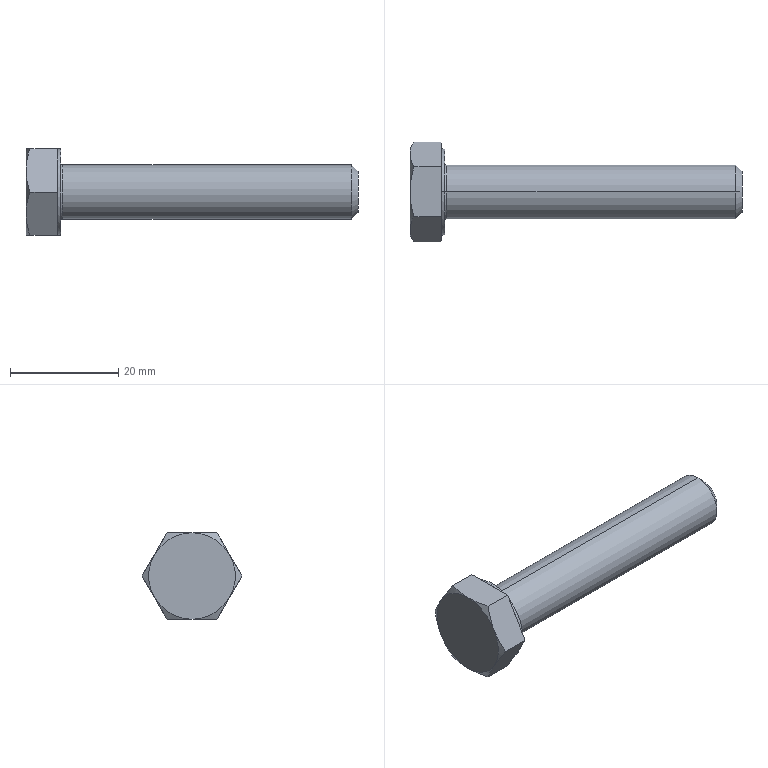Part | SolidWorks | features RevCut 4, Chamfer 1, Extrusion 1, Fillet 1, LPattern 1, Revolution 1 | 1 solid | 35 faces | box 61.4 x 18.475 x 16 mm | volume 5702 mm3 | plane 15 | cone 14 | cylinder 4 | torus 2 | commonest cylinder face diameters 10 x2 16 x2
STEP:
#1=CARTESIAN_POINT('',(6.8,0.,5.));
#2=VERTEX_POINT('',#1);
#3=CARTESIAN_POINT('',(6.8,0.,-5.));
#4=VERTEX_POINT('',#3);
#5=CARTESIAN_POINT('',(6.8,0.,0.));
#6=DIRECTION('',(1.,0.,0.));
#7=DIRECTION('',(0.,0.,-1.));
#8=AXIS2_PLACEMENT_3D('',#5,#6,#7);
#9=CIRCLE('',#8,5.);
#10=EDGE_CURVE('',#2,#4,#9,.T.);
#11=ORIENTED_EDGE('',*,*,#10,.F.);
#12=CARTESIAN_POINT('',(6.4,0.,5.4));
#13=VERTEX_POINT('',#12);
#14=CARTESIAN_POINT('',(6.8,0.,5.4));
#15=DIRECTION('',(0.,1.,0.));
#16=DIRECTION('',(0.,0.,1.));
#17=AXIS2_PLACEMENT_3D('',#14,#15,#16);
#18=CIRCLE('',#17,0.4);
#19=EDGE_CURVE('',#2,#13,#18,.T.);
#20=ORIENTED_EDGE('',*,*,#19,.T.);
#21=CARTESIAN_POINT('',(6.4,0.,-5.4));
#22=VERTEX_POINT('',#21);
#23=CARTESIAN_POINT('',(6.4,0.,0.));
#24=DIRECTION('',(-1.,0.,0.));
#25=DIRECTION('',(0.,0.,-1.));
#26=AXIS2_PLACEMENT_3D('',#23,#24,#25);
#27=CIRCLE('',#26,5.4);
#28=EDGE_CURVE('',#22,#13,#27,.T.);
#29=ORIENTED_EDGE('',*,*,#28,.F.);
#30=CARTESIAN_POINT('',(6.8,0.,-5.4));
#31=DIRECTION('',(0.,-1.,0.));
#32=DIRECTION('',(0.,0.,-1.));
#33=AXIS2_PLACEMENT_3D('',#30,#31,#32);
#34=CIRCLE('',#33,0.4);
#35=EDGE_CURVE('',#4,#22,#34,.T.);
#36=ORIENTED_EDGE('',*,*,#35,.F.);
#37=EDGE_LOOP('',(#11,#20,#29,#36));
#38=FACE_OUTER_BOUND('',#37,.T.);
#39=CARTESIAN_POINT('',(6.8,0.,0.));
#40=DIRECTION('',(1.,0.,0.));
#41=DIRECTION('',(0.,0.,-1.));
#42=AXIS2_PLACEMENT_3D('',#39,#40,#41);
#43=TOROIDAL_SURFACE('',#42,5.4,0.4);
#44=ADVANCED_FACE('',(#38),#43,.F.);
#45=CARTESIAN_POINT('',(61.4,0.,-3.8));
#46=VERTEX_POINT('',#45);
#47=CARTESIAN_POINT('',(61.4,0.,3.8));
#48=VERTEX_POINT('',#47);
#49=CARTESIAN_POINT('',(61.4,0.,0.));
#50=DIRECTION('',(1.,0.,0.));
#51=DIRECTION('',(0.,0.,1.));
#52=AXIS2_PLACEMENT_3D('',#49,#50,#51);
#53=CIRCLE('',#52,3.8);
#54=EDGE_CURVE('',#46,#48,#53,.T.);
#55=ORIENTED_EDGE('',*,*,#54,.F.);
#56=CARTESIAN_POINT('',(60.2,0.,-5.));
#57=VERTEX_POINT('',#56);
#58=CARTESIAN_POINT('',(60.2,0.,-5.));
#59=DIRECTION('',(-0.7071,0.,-0.7071));
#60=VECTOR('',#59,1000.);
#61=LINE('',#58,#60);
#62=EDGE_CURVE('',#46,#57,#61,.T.);
#63=ORIENTED_EDGE('',*,*,#62,.T.);
#64=CARTESIAN_POINT('',(60.2,0.,5.));
#65=VERTEX_POINT('',#64);
#66=CARTESIAN_POINT('',(60.2,0.,0.));
#67=DIRECTION('',(-1.,0.,0.));
#68=DIRECTION('',(0.,0.,1.));
#69=AXIS2_PLACEMENT_3D('',#66,#67,#68);
#70=CIRCLE('',#69,5.);
#71=EDGE_CURVE('',#65,#57,#70,.T.);
#72=ORIENTED_EDGE('',*,*,#71,.F.);
#73=CARTESIAN_POINT('',(60.2,0.,5.));
#74=DIRECTION('',(-0.7071,0.,0.7071));
#75=VECTOR('',#74,1000.);
#76=LINE('',#73,#75);
#77=EDGE_CURVE('',#48,#65,#76,.T.);
#78=ORIENTED_EDGE('',*,*,#77,.F.);
#79=EDGE_LOOP('',(#55,#63,#72,#78));
#80=FACE_OUTER_BOUND('',#79,.T.);
#81=CARTESIAN_POINT('',(60.2,0.,0.));
#82=DIRECTION('',(-1.,0.,0.));
#83=DIRECTION('',(0.,0.,1.));
#84=AXIS2_PLACEMENT_3D('',#81,#82,#83);
#85=CONICAL_SURFACE('',#84,5.,0.7854);
#86=ADVANCED_FACE('',(#80),#85,.T.);
#87=ORIENTED_EDGE('',*,*,#71,.T.);
#88=CARTESIAN_POINT('',(0.,0.,-5.));
#89=DIRECTION('',(-1.,0.,0.));
#90=VECTOR('',#89,1000.);
#91=LINE('',#88,#90);
#92=EDGE_CURVE('',#57,#4,#91,.T.);
#93=ORIENTED_EDGE('',*,*,#92,.T.);
#94=CARTESIAN_POINT('',(6.8,0.,0.));
#95=DIRECTION('',(1.,0.,0.));
#96=DIRECTION('',(0.,0.,-1.));
#97=AXIS2_PLACEMENT_3D('',#94,#95,#96);
#98=CIRCLE('',#97,5.);
#99=EDGE_CURVE('',#4,#2,#98,.T.);
#100=ORIENTED_EDGE('',*,*,#99,.T.);
#101=CARTESIAN_POINT('',(0.,0.,5.));
#102=DIRECTION('',(-1.,0.,0.));
#103=VECTOR('',#102,1000.);
#104=LINE('',#101,#103);
#105=EDGE_CURVE('',#65,#2,#104,.T.);
#106=ORIENTED_EDGE('',*,*,#105,.F.);
#107=EDGE_LOOP('',(#87,#93,#100,#106));
#108=FACE_OUTER_BOUND('',#107,.T.);
#109=CARTESIAN_POINT('',(0.,0.,0.));
#110=DIRECTION('',(-1.,0.,0.));
#111=DIRECTION('',(0.,0.,1.));
#112=AXIS2_PLACEMENT_3D('',#109,#110,#111);
#113=CYLINDRICAL_SURFACE('',#112,5.);
#114=ADVANCED_FACE('',(#108),#113,.T.);
#115=CARTESIAN_POINT('',(6.4,0.,-8.));
#116=VERTEX_POINT('',#115);
#117=CARTESIAN_POINT('',(6.4,0.,8.));
#118=VERTEX_POINT('',#117);
#119=CARTESIAN_POINT('',(6.4,0.,0.));
#120=DIRECTION('',(1.,0.,0.));
#121=DIRECTION('',(0.,0.,-1.));
#122=AXIS2_PLACEMENT_3D('',#119,#120,#121);
#123=CIRCLE('',#122,8.);
#124=EDGE_CURVE('',#116,#118,#123,.T.);
#125=ORIENTED_EDGE('',*,*,#124,.F.);
#126=CARTESIAN_POINT('',(5.8,0.,-8.));
#127=VERTEX_POINT('',#126);
#128=CARTESIAN_POINT('',(0.,0.,-8.));
#129=DIRECTION('',(-1.,0.,0.));
#130=VECTOR('',#129,1000.);
#131=LINE('',#128,#130);
#132=EDGE_CURVE('',#116,#127,#131,.T.);
#133=ORIENTED_EDGE('',*,*,#132,.T.);
#134=CARTESIAN_POINT('',(5.8,6.928,-4.));
#135=VERTEX_POINT('',#134);
#136=CARTESIAN_POINT('',(5.8,0.,0.));
#137=DIRECTION('',(-1.,0.,0.));
#138=DIRECTION('',(0.,0.,1.));
#139=AXIS2_PLACEMENT_3D('',#136,#137,#138);
#140=CIRCLE('',#139,8.);
#141=EDGE_CURVE('',#135,#127,#140,.T.);
#142=ORIENTED_EDGE('',*,*,#141,.F.);
#143=CARTESIAN_POINT('',(5.8,6.928,4.));
#144=VERTEX_POINT('',#143);
#145=CARTESIAN_POINT('',(5.8,0.,0.));
#146=DIRECTION('',(-1.,0.,0.));
#147=DIRECTION('',(0.,0.,1.));
#148=AXIS2_PLACEMENT_3D('',#145,#146,#147);
#149=CIRCLE('',#148,8.);
#150=EDGE_CURVE('',#144,#135,#149,.T.);
#151=ORIENTED_EDGE('',*,*,#150,.F.);
#152=CARTESIAN_POINT('',(5.8,0.,8.));
#153=VERTEX_POINT('',#152);
#154=CARTESIAN_POINT('',(5.8,0.,0.));
#155=DIRECTION('',(-1.,0.,0.));
#156=DIRECTION('',(0.,0.,1.));
#157=AXIS2_PLACEMENT_3D('',#154,#155,#156);
#158=CIRCLE('',#157,8.);
#159=EDGE_CURVE('',#153,#144,#158,.T.);
#160=ORIENTED_EDGE('',*,*,#159,.F.);
#161=CARTESIAN_POINT('',(0.,0.,8.));
#162=DIRECTION('',(-1.,0.,0.));
#163=VECTOR('',#162,1000.);
#164=LINE('',#161,#163);
#165=EDGE_CURVE('',#118,#153,#164,.T.);
#166=ORIENTED_EDGE('',*,*,#165,.F.);
#167=EDGE_LOOP('',(#125,#133,#142,#151,#160,#166));
#168=FACE_OUTER_BOUND('',#167,.T.);
#169=CARTESIAN_POINT('',(0.,0.,0.));
#170=DIRECTION('',(-1.,0.,0.));
#171=DIRECTION('',(0.,0.,1.));
#172=AXIS2_PLACEMENT_3D('',#169,#170,#171);
#173=CYLINDRICAL_SURFACE('',#172,8.);
#174=ADVANCED_FACE('',(#168),#173,.T.);
#175=CARTESIAN_POINT('',(5.8,4.824,-7.644));
#176=VERTEX_POINT('',#175);
#177=CARTESIAN_POINT('',(5.8,4.619,-8.));
#178=DIRECTION('',(0.,0.5,0.866));
#179=VECTOR('',#178,1000.);
#180=LINE('',#177,#179);
#181=EDGE_CURVE('',#176,#135,#180,.T.);
#182=ORIENTED_EDGE('',*,*,#181,.F.);
#183=CARTESIAN_POINT('',(5.685,4.619,-8.));
#184=VERTEX_POINT('',#183);
#185=CARTESIAN_POINT('',(5.685,4.619,-8.));
#186=CARTESIAN_POINT('',(5.725,4.687,-7.882));
#187=CARTESIAN_POINT('',(5.763,4.756,-7.763));
#188=CARTESIAN_POINT('',(5.8,4.824,-7.644));
#189=B_SPLINE_CURVE_WITH_KNOTS('',3,(#185,#186,#187,#188),.UNSPECIFIED.,.F.,.F.,(4,4),(0.000000238,0.0004231),.UNSPECIFIED.);
#190=EDGE_CURVE('',#184,#176,#189,.T.);
#191=ORIENTED_EDGE('',*,*,#190,.F.);
#192=CARTESIAN_POINT('',(0.7145,4.619,-8.));
#193=VERTEX_POINT('',#192);
#194=CARTESIAN_POINT('',(6.4,4.619,-8.));
#195=DIRECTION('',(-1.,0.,0.));
#196=VECTOR('',#195,1000.);
#197=LINE('',#194,#196);
#198=EDGE_CURVE('',#184,#193,#197,.T.);
#199=ORIENTED_EDGE('',*,*,#198,.T.);
#200=CARTESIAN_POINT('',(0.,6.928,-4.));
#201=VERTEX_POINT('',#200);
#202=CARTESIAN_POINT('',(0.,6.928,-4.));
#203=CARTESIAN_POINT('',(0.,6.732,-4.339));
#204=CARTESIAN_POINT('',(0.01689,6.535,-4.68));
#205=CARTESIAN_POINT('',(0.08225,6.146,-5.355));
#206=CARTESIAN_POINT('',(0.1307,5.952,-5.69));
#207=CARTESIAN_POINT('',(0.3174,5.376,-6.689));
#208=CARTESIAN_POINT('',(0.497,4.996,-7.347));
#209=CARTESIAN_POINT('',(0.7145,4.619,-8.));
#210=B_SPLINE_CURVE_WITH_KNOTS('',3,(#202,#203,#204,#205,#206,#207,#208,#209),.UNSPECIFIED.,.F.,.F.,(4,2,2,4),(0.004674,0.005838,0.007002,0.00933),.UNSPECIFIED.);
#211=EDGE_CURVE('',#201,#193,#210,.T.);
#212=ORIENTED_EDGE('',*,*,#211,.F.);
#213=CARTESIAN_POINT('',(0.7145,9.238,0.));
#214=VERTEX_POINT('',#213);
#215=CARTESIAN_POINT('',(0.7145,9.238,0.));
#216=CARTESIAN_POINT('',(0.4964,8.86,-0.6543));
#217=CARTESIAN_POINT('',(0.3167,8.479,-1.313));
#218=CARTESIAN_POINT('',(0.0681,7.71,-2.646));
#219=CARTESIAN_POINT('',(0.,7.322,-3.319));
#220=CARTESIAN_POINT('',(0.,6.928,-4.));
#221=B_SPLINE_CURVE_WITH_KNOTS('',3,(#215,#216,#217,#218,#219,#220),.UNSPECIFIED.,.F.,.F.,(4,2,4),(0.000000238,0.002337,0.004674),.UNSPECIFIED.);
#222=EDGE_CURVE('',#214,#201,#221,.T.);
#223=ORIENTED_EDGE('',*,*,#222,.F.);
#224=CARTESIAN_POINT('',(5.685,9.238,0.));
#225=VERTEX_POINT('',#224);
#226=CARTESIAN_POINT('',(6.4,9.238,0.));
#227=DIRECTION('',(-1.,0.,0.));
#228=VECTOR('',#227,1000.);
#229=LINE('',#226,#228);
#230=EDGE_CURVE('',#225,#214,#229,.T.);
#231=ORIENTED_EDGE('',*,*,#230,.F.);
#232=CARTESIAN_POINT('',(5.8,9.032,-0.3557));
#233=VERTEX_POINT('',#232);
#234=CARTESIAN_POINT('',(5.8,9.032,-0.3557));
#235=CARTESIAN_POINT('',(5.763,9.101,-0.237));
#236=CARTESIAN_POINT('',(5.725,9.169,-0.1184));
#237=CARTESIAN_POINT('',(5.685,9.238,0.));
#238=B_SPLINE_CURVE_WITH_KNOTS('',3,(#234,#235,#236,#237),.UNSPECIFIED.,.F.,.F.,(4,4),(0.008907,0.00933),.UNSPECIFIED.);
#239=EDGE_CURVE('',#233,#225,#238,.T.);
#240=ORIENTED_EDGE('',*,*,#239,.F.);
#241=CARTESIAN_POINT('',(5.8,4.619,-8.));
#242=DIRECTION('',(0.,0.5,0.866));
#243=VECTOR('',#242,1000.);
#244=LINE('',#241,#243);
#245=EDGE_CURVE('',#135,#233,#244,.T.);
#246=ORIENTED_EDGE('',*,*,#245,.F.);
#247=EDGE_LOOP('',(#182,#191,#199,#212,#223,#231,#240,#246));
#248=FACE_OUTER_BOUND('',#247,.T.);
#249=CARTESIAN_POINT('',(6.4,4.619,-8.));
#250=DIRECTION('',(0.,-0.866,0.5));
#251=DIRECTION('',(0.,-0.5,-0.866));
#252=AXIS2_PLACEMENT_3D('',#249,#250,#251);
#253=PLANE('',#252);
#254=ADVANCED_FACE('',(#248),#253,.F.);
#255=CARTESIAN_POINT('',(5.8,9.032,0.3557));
#256=VERTEX_POINT('',#255);
#257=CARTESIAN_POINT('',(5.8,9.238,0.));
#258=DIRECTION('',(0.,-0.5,0.866));
#259=VECTOR('',#258,1000.);
#260=LINE('',#257,#259);
#261=EDGE_CURVE('',#256,#144,#260,.T.);
#262=ORIENTED_EDGE('',*,*,#261,.F.);
#263=CARTESIAN_POINT('',(5.685,9.238,0.));
#264=CARTESIAN_POINT('',(5.725,9.169,0.1184));
#265=CARTESIAN_POINT('',(5.763,9.101,0.237));
#266=CARTESIAN_POINT('',(5.8,9.032,0.3557));
#267=B_SPLINE_CURVE_WITH_KNOTS('',3,(#263,#264,#265,#266),.UNSPECIFIED.,.F.,.F.,(4,4),(0.000000238,0.0004231),.UNSPECIFIED.);
#268=EDGE_CURVE('',#225,#256,#267,.T.);
#269=ORIENTED_EDGE('',*,*,#268,.F.);
#270=ORIENTED_EDGE('',*,*,#230,.T.);
#271=CARTESIAN_POINT('',(0.,6.928,4.));
#272=VERTEX_POINT('',#271);
#273=CARTESIAN_POINT('',(0.,6.928,4.));
#274=CARTESIAN_POINT('',(0.,7.124,3.661));
#275=CARTESIAN_POINT('',(0.01689,7.321,3.32));
#276=CARTESIAN_POINT('',(0.08225,7.711,2.645));
#277=CARTESIAN_POINT('',(0.1307,7.904,2.31));
#278=CARTESIAN_POINT('',(0.3174,8.481,1.311));
#279=CARTESIAN_POINT('',(0.497,8.861,0.6527));
#280=CARTESIAN_POINT('',(0.7145,9.238,0.));
#281=B_SPLINE_CURVE_WITH_KNOTS('',3,(#273,#274,#275,#276,#277,#278,#279,#280),.UNSPECIFIED.,.F.,.F.,(4,2,2,4),(0.004674,0.005838,0.007002,0.00933),.UNSPECIFIED.);
#282=EDGE_CURVE('',#272,#214,#281,.T.);
#283=ORIENTED_EDGE('',*,*,#282,.F.);
#284=CARTESIAN_POINT('',(0.7145,4.619,8.));
#285=VERTEX_POINT('',#284);
#286=CARTESIAN_POINT('',(0.7145,4.619,8.));
#287=CARTESIAN_POINT('',(0.4964,4.997,7.346));
#288=CARTESIAN_POINT('',(0.3167,5.377,6.687));
#289=CARTESIAN_POINT('',(0.0681,6.146,5.354));
#290=CARTESIAN_POINT('',(0.,6.535,4.681));
#291=CARTESIAN_POINT('',(0.,6.928,4.));
#292=B_SPLINE_CURVE_WITH_KNOTS('',3,(#286,#287,#288,#289,#290,#291),.UNSPECIFIED.,.F.,.F.,(4,2,4),(0.000000238,0.002337,0.004674),.UNSPECIFIED.);
#293=EDGE_CURVE('',#285,#272,#292,.T.);
#294=ORIENTED_EDGE('',*,*,#293,.F.);
#295=CARTESIAN_POINT('',(5.685,4.619,8.));
#296=VERTEX_POINT('',#295);
#297=CARTESIAN_POINT('',(6.4,4.619,8.));
#298=DIRECTION('',(-1.,0.,0.));
#299=VECTOR('',#298,1000.);
#300=LINE('',#297,#299);
#301=EDGE_CURVE('',#296,#285,#300,.T.);
#302=ORIENTED_EDGE('',*,*,#301,.F.);
#303=CARTESIAN_POINT('',(5.8,4.824,7.644));
#304=VERTEX_POINT('',#303);
#305=CARTESIAN_POINT('',(5.8,4.824,7.644));
#306=CARTESIAN_POINT('',(5.763,4.756,7.763));
#307=CARTESIAN_POINT('',(5.725,4.687,7.882));
#308=CARTESIAN_POINT('',(5.685,4.619,8.));
#309=B_SPLINE_CURVE_WITH_KNOTS('',3,(#305,#306,#307,#308),.UNSPECIFIED.,.F.,.F.,(4,4),(0.008907,0.00933),.UNSPECIFIED.);
#310=EDGE_CURVE('',#304,#296,#309,.T.);
#311=ORIENTED_EDGE('',*,*,#310,.F.);
#312=CARTESIAN_POINT('',(5.8,9.238,0.));
#313=DIRECTION('',(0.,-0.5,0.866));
#314=VECTOR('',#313,1000.);
#315=LINE('',#312,#314);
#316=EDGE_CURVE('',#144,#304,#315,.T.);
#317=ORIENTED_EDGE('',*,*,#316,.F.);
#318=EDGE_LOOP('',(#262,#269,#270,#283,#294,#302,#311,#317));
#319=FACE_OUTER_BOUND('',#318,.T.);
#320=CARTESIAN_POINT('',(6.4,9.238,0.));
#321=DIRECTION('',(0.,-0.866,-0.5));
#322=DIRECTION('',(0.,0.5,-0.866));
#323=AXIS2_PLACEMENT_3D('',#320,#321,#322);
#324=PLANE('',#323);
#325=ADVANCED_FACE('',(#319),#324,.F.);
#326=CARTESIAN_POINT('',(5.8,4.208,8.));
#327=VERTEX_POINT('',#326);
#328=CARTESIAN_POINT('',(5.8,4.619,8.));
#329=DIRECTION('',(0.,-1.,0.));
#330=VECTOR('',#329,1000.);
#331=LINE('',#328,#330);
#332=EDGE_CURVE('',#327,#153,#331,.T.);
#333=ORIENTED_EDGE('',*,*,#332,.F.);
#334=CARTESIAN_POINT('',(5.685,4.619,8.));
#335=CARTESIAN_POINT('',(5.725,4.482,8.));
#336=CARTESIAN_POINT('',(5.763,4.345,8.));
#337=CARTESIAN_POINT('',(5.8,4.208,8.));
#338=B_SPLINE_CURVE_WITH_KNOTS('',3,(#334,#335,#336,#337),.UNSPECIFIED.,.F.,.F.,(4,4),(0.02285,0.02328),.UNSPECIFIED.);
#339=EDGE_CURVE('',#296,#327,#338,.T.);
#340=ORIENTED_EDGE('',*,*,#339,.F.);
#341=ORIENTED_EDGE('',*,*,#301,.T.);
#342=CARTESIAN_POINT('',(0.,0.,8.));
#343=VERTEX_POINT('',#342);
#344=CARTESIAN_POINT('',(0.,0.,8.));
#345=CARTESIAN_POINT('',(0.,0.3913,8.));
#346=CARTESIAN_POINT('',(0.01678,0.7854,8.));
#347=CARTESIAN_POINT('',(0.08286,1.571,8.));
#348=CARTESIAN_POINT('',(0.1318,1.96,8.));
#349=CARTESIAN_POINT('',(0.3194,3.115,8.));
#350=CARTESIAN_POINT('',(0.4988,3.872,8.));
#351=CARTESIAN_POINT('',(0.7145,4.619,8.));
#352=B_SPLINE_CURVE_WITH_KNOTS('',3,(#344,#345,#346,#347,#348,#349,#350,#351),.UNSPECIFIED.,.F.,.F.,(4,2,2,4),(0.01337,0.01454,0.01571,0.01805),.UNSPECIFIED.);
#353=EDGE_CURVE('',#343,#285,#352,.T.);
#354=ORIENTED_EDGE('',*,*,#353,.F.);
#355=CARTESIAN_POINT('',(0.7145,-4.619,8.));
#356=VERTEX_POINT('',#355);
#357=CARTESIAN_POINT('',(0.7145,-4.619,8.));
#358=CARTESIAN_POINT('',(0.4973,-3.866,8.));
#359=CARTESIAN_POINT('',(0.3158,-3.098,8.));
#360=CARTESIAN_POINT('',(0.0673,-1.557,8.));
#361=CARTESIAN_POINT('',(0.,-0.7819,8.));
#362=CARTESIAN_POINT('',(0.,0.,8.));
#363=B_SPLINE_CURVE_WITH_KNOTS('',3,(#357,#358,#359,#360,#361,#362),.UNSPECIFIED.,.F.,.F.,(4,2,4),(0.00869,0.01103,0.01337),.UNSPECIFIED.);
#364=EDGE_CURVE('',#356,#343,#363,.T.);
#365=ORIENTED_EDGE('',*,*,#364,.F.);
#366=CARTESIAN_POINT('',(5.685,-4.619,8.));
#367=VERTEX_POINT('',#366);
#368=CARTESIAN_POINT('',(6.4,-4.619,8.));
#369=DIRECTION('',(-1.,0.,0.));
#370=VECTOR('',#369,1000.);
#371=LINE('',#368,#370);
#372=EDGE_CURVE('',#367,#356,#371,.T.);
#373=ORIENTED_EDGE('',*,*,#372,.F.);
#374=CARTESIAN_POINT('',(5.8,-4.208,8.));
#375=VERTEX_POINT('',#374);
#376=CARTESIAN_POINT('',(5.8,-4.208,8.));
#377=CARTESIAN_POINT('',(5.763,-4.345,8.));
#378=CARTESIAN_POINT('',(5.725,-4.482,8.));
#379=CARTESIAN_POINT('',(5.685,-4.619,8.));
#380=B_SPLINE_CURVE_WITH_KNOTS('',3,(#376,#377,#378,#379),.UNSPECIFIED.,.F.,.F.,(4,4),(0.03178,0.03221),.UNSPECIFIED.);
#381=EDGE_CURVE('',#375,#367,#380,.T.);
#382=ORIENTED_EDGE('',*,*,#381,.F.);
#383=CARTESIAN_POINT('',(5.8,4.619,8.));
#384=DIRECTION('',(0.,-1.,0.));
#385=VECTOR('',#384,1000.);
#386=LINE('',#383,#385);
#387=EDGE_CURVE('',#153,#375,#386,.T.);
#388=ORIENTED_EDGE('',*,*,#387,.F.);
#389=EDGE_LOOP('',(#333,#340,#341,#354,#365,#373,#382,#388));
#390=FACE_OUTER_BOUND('',#389,.T.);
#391=CARTESIAN_POINT('',(6.4,4.619,8.));
#392=DIRECTION('',(0.,0.,-1.));
#393=DIRECTION('',(-1.,0.,0.));
#394=AXIS2_PLACEMENT_3D('',#391,#392,#393);
#395=PLANE('',#394);
#396=ADVANCED_FACE('',(#390),#395,.F.);
#397=CARTESIAN_POINT('',(5.8,-4.824,7.644));
#398=VERTEX_POINT('',#397);
#399=CARTESIAN_POINT('',(5.8,-6.928,4.));
#400=VERTEX_POINT('',#399);
#401=CARTESIAN_POINT('',(5.8,-9.238,0.));
#402=DIRECTION('',(0.,-0.5,-0.866));
#403=VECTOR('',#402,1000.);
#404=LINE('',#401,#403);
#405=EDGE_CURVE('',#398,#400,#404,.T.);
#406=ORIENTED_EDGE('',*,*,#405,.F.);
#407=CARTESIAN_POINT('',(5.685,-4.619,8.));
#408=CARTESIAN_POINT('',(5.725,-4.687,7.882));
#409=CARTESIAN_POINT('',(5.763,-4.756,7.763));
#410=CARTESIAN_POINT('',(5.8,-4.824,7.644));
#411=B_SPLINE_CURVE_WITH_KNOTS('',3,(#407,#408,#409,#410),.UNSPECIFIED.,.F.,.F.,(4,4),(0.000000238,0.0004231),.UNSPECIFIED.);
#412=EDGE_CURVE('',#367,#398,#411,.T.);
#413=ORIENTED_EDGE('',*,*,#412,.F.);
#414=ORIENTED_EDGE('',*,*,#372,.T.);
#415=CARTESIAN_POINT('',(0.,-6.928,4.));
#416=VERTEX_POINT('',#415);
#417=CARTESIAN_POINT('',(0.,-6.928,4.));
#418=CARTESIAN_POINT('',(0.,-6.732,4.339));
#419=CARTESIAN_POINT('',(0.01689,-6.535,4.68));
#420=CARTESIAN_POINT('',(0.08225,-6.146,5.355));
#421=CARTESIAN_POINT('',(0.1307,-5.952,5.69));
#422=CARTESIAN_POINT('',(0.3174,-5.376,6.689));
#423=CARTESIAN_POINT('',(0.497,-4.996,7.347));
#424=CARTESIAN_POINT('',(0.7145,-4.619,8.));
#425=B_SPLINE_CURVE_WITH_KNOTS('',3,(#417,#418,#419,#420,#421,#422,#423,#424),.UNSPECIFIED.,.F.,.F.,(4,2,2,4),(0.004674,0.005838,0.007002,0.00933),.UNSPECIFIED.);
#426=EDGE_CURVE('',#416,#356,#425,.T.);
#427=ORIENTED_EDGE('',*,*,#426,.F.);
#428=CARTESIAN_POINT('',(0.7145,-9.238,0.));
#429=VERTEX_POINT('',#428);
#430=CARTESIAN_POINT('',(0.7145,-9.238,0.));
#431=CARTESIAN_POINT('',(0.4964,-8.86,0.6543));
#432=CARTESIAN_POINT('',(0.3167,-8.479,1.313));
#433=CARTESIAN_POINT('',(0.0681,-7.71,2.646));
#434=CARTESIAN_POINT('',(0.,-7.322,3.319));
#435=CARTESIAN_POINT('',(0.,-6.928,4.));
#436=B_SPLINE_CURVE_WITH_KNOTS('',3,(#430,#431,#432,#433,#434,#435),.UNSPECIFIED.,.F.,.F.,(4,2,4),(0.000000238,0.002337,0.004674),.UNSPECIFIED.);
#437=EDGE_CURVE('',#429,#416,#436,.T.);
#438=ORIENTED_EDGE('',*,*,#437,.F.);
#439=CARTESIAN_POINT('',(5.685,-9.238,0.));
#440=VERTEX_POINT('',#439);
#441=CARTESIAN_POINT('',(6.4,-9.238,0.));
#442=DIRECTION('',(-1.,0.,0.));
#443=VECTOR('',#442,1000.);
#444=LINE('',#441,#443);
#445=EDGE_CURVE('',#440,#429,#444,.T.);
#446=ORIENTED_EDGE('',*,*,#445,.F.);
#447=CARTESIAN_POINT('',(5.8,-9.032,0.3557));
#448=VERTEX_POINT('',#447);
#449=CARTESIAN_POINT('',(5.8,-9.032,0.3557));
#450=CARTESIAN_POINT('',(5.763,-9.101,0.237));
#451=CARTESIAN_POINT('',(5.725,-9.169,0.1184));
#452=CARTESIAN_POINT('',(5.685,-9.238,0.));
#453=B_SPLINE_CURVE_WITH_KNOTS('',3,(#449,#450,#451,#452),.UNSPECIFIED.,.F.,.F.,(4,4),(0.008907,0.00933),.UNSPECIFIED.);
#454=EDGE_CURVE('',#448,#440,#453,.T.);
#455=ORIENTED_EDGE('',*,*,#454,.F.);
#456=CARTESIAN_POINT('',(5.8,-9.238,0.));
#457=DIRECTION('',(0.,-0.5,-0.866));
#458=VECTOR('',#457,1000.);
#459=LINE('',#456,#458);
#460=EDGE_CURVE('',#400,#448,#459,.T.);
#461=ORIENTED_EDGE('',*,*,#460,.F.);
#462=EDGE_LOOP('',(#406,#413,#414,#427,#438,#446,#455,#461));
#463=FACE_OUTER_BOUND('',#462,.T.);
#464=CARTESIAN_POINT('',(6.4,-9.238,0.));
#465=DIRECTION('',(0.,0.866,-0.5));
#466=DIRECTION('',(0.,0.5,0.866));
#467=AXIS2_PLACEMENT_3D('',#464,#465,#466);
#468=PLANE('',#467);
#469=ADVANCED_FACE('',(#463),#468,.F.);
#470=CARTESIAN_POINT('',(5.8,-9.032,-0.3557));
#471=VERTEX_POINT('',#470);
#472=CARTESIAN_POINT('',(5.8,-6.928,-4.));
#473=VERTEX_POINT('',#472);
#474=CARTESIAN_POINT('',(5.8,-4.619,-8.));
#475=DIRECTION('',(0.,0.5,-0.866));
#476=VECTOR('',#475,1000.);
#477=LINE('',#474,#476);
#478=EDGE_CURVE('',#471,#473,#477,.T.);
#479=ORIENTED_EDGE('',*,*,#478,.F.);
#480=CARTESIAN_POINT('',(5.685,-9.238,0.));
#481=CARTESIAN_POINT('',(5.725,-9.169,-0.1184));
#482=CARTESIAN_POINT('',(5.763,-9.101,-0.237));
#483=CARTESIAN_POINT('',(5.8,-9.032,-0.3557));
#484=B_SPLINE_CURVE_WITH_KNOTS('',3,(#480,#481,#482,#483),.UNSPECIFIED.,.F.,.F.,(4,4),(0.000000238,0.0004231),.UNSPECIFIED.);
#485=EDGE_CURVE('',#440,#471,#484,.T.);
#486=ORIENTED_EDGE('',*,*,#485,.F.);
#487=ORIENTED_EDGE('',*,*,#445,.T.);
#488=CARTESIAN_POINT('',(0.,-6.928,-4.));
#489=VERTEX_POINT('',#488);
#490=CARTESIAN_POINT('',(0.,-6.928,-4.));
#491=CARTESIAN_POINT('',(0.,-7.124,-3.661));
#492=CARTESIAN_POINT('',(0.01689,-7.321,-3.32));
#493=CARTESIAN_POINT('',(0.08225,-7.711,-2.645));
#494=CARTESIAN_POINT('',(0.1307,-7.904,-2.31));
#495=CARTESIAN_POINT('',(0.3174,-8.481,-1.311));
#496=CARTESIAN_POINT('',(0.497,-8.861,-0.6527));
#497=CARTESIAN_POINT('',(0.7145,-9.238,0.));
#498=B_SPLINE_CURVE_WITH_KNOTS('',3,(#490,#491,#492,#493,#494,#495,#496,#497),.UNSPECIFIED.,.F.,.F.,(4,2,2,4),(0.004674,0.005838,0.007002,0.00933),.UNSPECIFIED.);
#499=EDGE_CURVE('',#489,#429,#498,.T.);
#500=ORIENTED_EDGE('',*,*,#499,.F.);
#501=CARTESIAN_POINT('',(0.7145,-4.619,-8.));
#502=VERTEX_POINT('',#501);
#503=CARTESIAN_POINT('',(0.7145,-4.619,-8.));
#504=CARTESIAN_POINT('',(0.4964,-4.997,-7.346));
#505=CARTESIAN_POINT('',(0.3167,-5.377,-6.687));
#506=CARTESIAN_POINT('',(0.0681,-6.146,-5.354));
#507=CARTESIAN_POINT('',(0.,-6.535,-4.681));
#508=CARTESIAN_POINT('',(0.,-6.928,-4.));
#509=B_SPLINE_CURVE_WITH_KNOTS('',3,(#503,#504,#505,#506,#507,#508),.UNSPECIFIED.,.F.,.F.,(4,2,4),(0.000000238,0.002337,0.004674),.UNSPECIFIED.);
#510=EDGE_CURVE('',#502,#489,#509,.T.);
#511=ORIENTED_EDGE('',*,*,#510,.F.);
#512=CARTESIAN_POINT('',(5.685,-4.619,-8.));
#513=VERTEX_POINT('',#512);
#514=CARTESIAN_POINT('',(6.4,-4.619,-8.));
#515=DIRECTION('',(-1.,0.,0.));
#516=VECTOR('',#515,1000.);
#517=LINE('',#514,#516);
#518=EDGE_CURVE('',#513,#502,#517,.T.);
#519=ORIENTED_EDGE('',*,*,#518,.F.);
#520=CARTESIAN_POINT('',(5.8,-4.824,-7.644));
#521=VERTEX_POINT('',#520);
#522=CARTESIAN_POINT('',(5.8,-4.824,-7.644));
#523=CARTESIAN_POINT('',(5.763,-4.756,-7.763));
#524=CARTESIAN_POINT('',(5.725,-4.687,-7.882));
#525=CARTESIAN_POINT('',(5.685,-4.619,-8.));
#526=B_SPLINE_CURVE_WITH_KNOTS('',3,(#522,#523,#524,#525),.UNSPECIFIED.,.F.,.F.,(4,4),(0.008907,0.00933),.UNSPECIFIED.);
#527=EDGE_CURVE('',#521,#513,#526,.T.);
#528=ORIENTED_EDGE('',*,*,#527,.F.);
#529=CARTESIAN_POINT('',(5.8,-4.619,-8.));
#530=DIRECTION('',(0.,0.5,-0.866));
#531=VECTOR('',#530,1000.);
#532=LINE('',#529,#531);
#533=EDGE_CURVE('',#473,#521,#532,.T.);
#534=ORIENTED_EDGE('',*,*,#533,.F.);
#535=EDGE_LOOP('',(#479,#486,#487,#500,#511,#519,#528,#534));
#536=FACE_OUTER_BOUND('',#535,.T.);
#537=CARTESIAN_POINT('',(6.4,-4.619,-8.));
#538=DIRECTION('',(0.,0.866,0.5));
#539=DIRECTION('',(0.,-0.5,0.866));
#540=AXIS2_PLACEMENT_3D('',#537,#538,#539);
#541=PLANE('',#540);
#542=ADVANCED_FACE('',(#536),#541,.F.);
#543=CARTESIAN_POINT('',(5.8,-4.208,-8.));
#544=VERTEX_POINT('',#543);
#545=CARTESIAN_POINT('',(5.8,4.619,-8.));
#546=DIRECTION('',(0.,1.,0.));
#547=VECTOR('',#546,1000.);
#548=LINE('',#545,#547);
#549=EDGE_CURVE('',#544,#127,#548,.T.);
#550=ORIENTED_EDGE('',*,*,#549,.F.);
#551=CARTESIAN_POINT('',(5.685,-4.619,-8.));
#552=CARTESIAN_POINT('',(5.725,-4.482,-8.));
#553=CARTESIAN_POINT('',(5.763,-4.345,-8.));
#554=CARTESIAN_POINT('',(5.8,-4.208,-8.));
#555=B_SPLINE_CURVE_WITH_KNOTS('',3,(#551,#552,#553,#554),.UNSPECIFIED.,.F.,.F.,(4,4),(0.00869,0.009114),.UNSPECIFIED.);
#556=EDGE_CURVE('',#513,#544,#555,.T.);
#557=ORIENTED_EDGE('',*,*,#556,.F.);
#558=ORIENTED_EDGE('',*,*,#518,.T.);
#559=CARTESIAN_POINT('',(0.,0.,-8.));
#560=VERTEX_POINT('',#559);
#561=CARTESIAN_POINT('',(0.,0.,-8.));
#562=CARTESIAN_POINT('',(0.,-0.7819,-8.));
#563=CARTESIAN_POINT('',(0.0673,-1.557,-8.));
#564=CARTESIAN_POINT('',(0.3158,-3.098,-8.));
#565=CARTESIAN_POINT('',(0.4973,-3.866,-8.));
#566=CARTESIAN_POINT('',(0.7145,-4.619,-8.));
#567=B_SPLINE_CURVE_WITH_KNOTS('',3,(#561,#562,#563,#564,#565,#566),.UNSPECIFIED.,.F.,.F.,(4,2,4),(0.02753,0.02987,0.03221),.UNSPECIFIED.);
#568=EDGE_CURVE('',#560,#502,#567,.T.);
#569=ORIENTED_EDGE('',*,*,#568,.F.);
#570=CARTESIAN_POINT('',(0.7145,4.619,-8.));
#571=CARTESIAN_POINT('',(0.4988,3.872,-8.));
#572=CARTESIAN_POINT('',(0.3194,3.115,-8.));
#573=CARTESIAN_POINT('',(0.1318,1.96,-8.));
#574=CARTESIAN_POINT('',(0.08286,1.571,-8.));
#575=CARTESIAN_POINT('',(0.01678,0.7854,-8.));
#576=CARTESIAN_POINT('',(0.,0.3913,-8.));
#577=CARTESIAN_POINT('',(0.,0.,-8.));
#578=B_SPLINE_CURVE_WITH_KNOTS('',3,(#570,#571,#572,#573,#574,#575,#576,#577),.UNSPECIFIED.,.F.,.F.,(4,2,2,4),(0.02285,0.02519,0.02636,0.02753),.UNSPECIFIED.);
#579=EDGE_CURVE('',#193,#560,#578,.T.);
#580=ORIENTED_EDGE('',*,*,#579,.F.);
#581=ORIENTED_EDGE('',*,*,#198,.F.);
#582=CARTESIAN_POINT('',(5.8,4.208,-8.));
#583=VERTEX_POINT('',#582);
#584=CARTESIAN_POINT('',(5.8,4.208,-8.));
#585=CARTESIAN_POINT('',(5.763,4.345,-8.));
#586=CARTESIAN_POINT('',(5.725,4.482,-8.));
#587=CARTESIAN_POINT('',(5.685,4.619,-8.));
#588=B_SPLINE_CURVE_WITH_KNOTS('',3,(#584,#585,#586,#587),.UNSPECIFIED.,.F.,.F.,(4,4),(0.01762,0.01805),.UNSPECIFIED.);
#589=EDGE_CURVE('',#583,#184,#588,.T.);
#590=ORIENTED_EDGE('',*,*,#589,.F.);
#591=CARTESIAN_POINT('',(5.8,4.619,-8.));
#592=DIRECTION('',(0.,1.,0.));
#593=VECTOR('',#592,1000.);
#594=LINE('',#591,#593);
#595=EDGE_CURVE('',#127,#583,#594,.T.);
#596=ORIENTED_EDGE('',*,*,#595,.F.);
#597=EDGE_LOOP('',(#550,#557,#558,#569,#580,#581,#590,#596));
#598=FACE_OUTER_BOUND('',#597,.T.);
#599=CARTESIAN_POINT('',(6.4,4.619,-8.));
#600=DIRECTION('',(0.,0.,1.));
#601=DIRECTION('',(0.,-1.,0.));
#602=AXIS2_PLACEMENT_3D('',#599,#600,#601);
#603=PLANE('',#602);
#604=ADVANCED_FACE('',(#598),#603,.F.);
#605=ORIENTED_EDGE('',*,*,#556,.T.);
#606=CARTESIAN_POINT('',(5.8,0.,0.));
#607=DIRECTION('',(-1.,0.,0.));
#608=DIRECTION('',(0.,0.,-1.));
#609=AXIS2_PLACEMENT_3D('',#606,#607,#608);
#610=CIRCLE('',#609,9.039);
#611=EDGE_CURVE('',#544,#521,#610,.T.);
#612=ORIENTED_EDGE('',*,*,#611,.T.);
#613=ORIENTED_EDGE('',*,*,#527,.T.);
#614=EDGE_LOOP('',(#605,#612,#613));
#615=FACE_OUTER_BOUND('',#614,.T.);
#616=CARTESIAN_POINT('',(2.799,0.,0.));
#617=DIRECTION('',(-1.,0.,0.));
#618=DIRECTION('',(0.,0.,1.));
#619=AXIS2_PLACEMENT_3D('',#616,#617,#618);
#620=CONICAL_SURFACE('',#619,14.238,1.047);
#621=ADVANCED_FACE('',(#615),#620,.T.);
#622=ORIENTED_EDGE('',*,*,#485,.T.);
#623=CARTESIAN_POINT('',(5.8,0.,0.));
#624=DIRECTION('',(-1.,0.,0.));
#625=DIRECTION('',(0.,0.,-1.));
#626=AXIS2_PLACEMENT_3D('',#623,#624,#625);
#627=CIRCLE('',#626,9.039);
#628=EDGE_CURVE('',#471,#448,#627,.T.);
#629=ORIENTED_EDGE('',*,*,#628,.T.);
#630=ORIENTED_EDGE('',*,*,#454,.T.);
#631=EDGE_LOOP('',(#622,#629,#630));
#632=FACE_OUTER_BOUND('',#631,.T.);
#633=CARTESIAN_POINT('',(2.799,0.,0.));
#634=DIRECTION('',(-1.,0.,0.));
#635=DIRECTION('',(0.,0.,1.));
#636=AXIS2_PLACEMENT_3D('',#633,#634,#635);
#637=CONICAL_SURFACE('',#636,14.238,1.047);
#638=ADVANCED_FACE('',(#632),#637,.T.);
#639=ORIENTED_EDGE('',*,*,#412,.T.);
#640=CARTESIAN_POINT('',(5.8,0.,0.));
#641=DIRECTION('',(-1.,0.,0.));
#642=DIRECTION('',(0.,0.,-1.));
#643=AXIS2_PLACEMENT_3D('',#640,#641,#642);
#644=CIRCLE('',#643,9.039);
#645=EDGE_CURVE('',#398,#375,#644,.T.);
#646=ORIENTED_EDGE('',*,*,#645,.T.);
#647=ORIENTED_EDGE('',*,*,#381,.T.);
#648=EDGE_LOOP('',(#639,#646,#647));
#649=FACE_OUTER_BOUND('',#648,.T.);
#650=CARTESIAN_POINT('',(2.799,0.,0.));
#651=DIRECTION('',(-1.,0.,0.));
#652=DIRECTION('',(0.,0.,1.));
#653=AXIS2_PLACEMENT_3D('',#650,#651,#652);
#654=CONICAL_SURFACE('',#653,14.238,1.047);
#655=ADVANCED_FACE('',(#649),#654,.T.);
#656=ORIENTED_EDGE('',*,*,#339,.T.);
#657=CARTESIAN_POINT('',(5.8,0.,0.));
#658=DIRECTION('',(-1.,0.,0.));
#659=DIRECTION('',(0.,0.,-1.));
#660=AXIS2_PLACEMENT_3D('',#657,#658,#659);
#661=CIRCLE('',#660,9.039);
#662=EDGE_CURVE('',#327,#304,#661,.T.);
#663=ORIENTED_EDGE('',*,*,#662,.T.);
#664=ORIENTED_EDGE('',*,*,#310,.T.);
#665=EDGE_LOOP('',(#656,#663,#664));
#666=FACE_OUTER_BOUND('',#665,.T.);
#667=CARTESIAN_POINT('',(2.799,0.,0.));
#668=DIRECTION('',(-1.,0.,0.));
#669=DIRECTION('',(0.,0.,1.));
#670=AXIS2_PLACEMENT_3D('',#667,#668,#669);
#671=CONICAL_SURFACE('',#670,14.238,1.047);
#672=ADVANCED_FACE('',(#666),#671,.T.);
#673=ORIENTED_EDGE('',*,*,#268,.T.);
#674=CARTESIAN_POINT('',(5.8,0.,0.));
#675=DIRECTION('',(-1.,0.,0.));
#676=DIRECTION('',(0.,0.,-1.));
#677=AXIS2_PLACEMENT_3D('',#674,#675,#676);
#678=CIRCLE('',#677,9.039);
#679=EDGE_CURVE('',#256,#233,#678,.T.);
#680=ORIENTED_EDGE('',*,*,#679,.T.);
#681=ORIENTED_EDGE('',*,*,#239,.T.);
#682=EDGE_LOOP('',(#673,#680,#681));
#683=FACE_OUTER_BOUND('',#682,.T.);
#684=CARTESIAN_POINT('',(2.799,0.,0.));
#685=DIRECTION('',(-1.,0.,0.));
#686=DIRECTION('',(0.,0.,1.));
#687=AXIS2_PLACEMENT_3D('',#684,#685,#686);
#688=CONICAL_SURFACE('',#687,14.238,1.047);
#689=ADVANCED_FACE('',(#683),#688,.T.);
#690=ORIENTED_EDGE('',*,*,#190,.T.);
#691=CARTESIAN_POINT('',(5.8,0.,0.));
#692=DIRECTION('',(-1.,0.,0.));
#693=DIRECTION('',(0.,0.,-1.));
#694=AXIS2_PLACEMENT_3D('',#691,#692,#693);
#695=CIRCLE('',#694,9.039);
#696=EDGE_CURVE('',#176,#583,#695,.T.);
#697=ORIENTED_EDGE('',*,*,#696,.T.);
#698=ORIENTED_EDGE('',*,*,#589,.T.);
#699=EDGE_LOOP('',(#690,#697,#698));
#700=FACE_OUTER_BOUND('',#699,.T.);
#701=CARTESIAN_POINT('',(2.799,0.,0.));
#702=DIRECTION('',(-1.,0.,0.));
#703=DIRECTION('',(0.,0.,1.));
#704=AXIS2_PLACEMENT_3D('',#701,#702,#703);
#705=CONICAL_SURFACE('',#704,14.238,1.047);
#706=ADVANCED_FACE('',(#700),#705,.T.);
#707=ORIENTED_EDGE('',*,*,#510,.T.);
#708=CARTESIAN_POINT('',(0.,0.,0.));
#709=DIRECTION('',(1.,0.,0.));
#710=DIRECTION('',(0.,0.,-1.));
#711=AXIS2_PLACEMENT_3D('',#708,#709,#710);
#712=CIRCLE('',#711,8.);
#713=EDGE_CURVE('',#489,#560,#712,.T.);
#714=ORIENTED_EDGE('',*,*,#713,.T.);
#715=ORIENTED_EDGE('',*,*,#568,.T.);
#716=EDGE_LOOP('',(#707,#714,#715));
#717=FACE_OUTER_BOUND('',#716,.T.);
#718=CARTESIAN_POINT('',(0.,0.,0.));
#719=DIRECTION('',(1.,0.,0.));
#720=DIRECTION('',(0.,0.,-1.));
#721=AXIS2_PLACEMENT_3D('',#718,#719,#720);
#722=CONICAL_SURFACE('',#721,8.,1.047);
#723=ADVANCED_FACE('',(#717),#722,.T.);
#724=ORIENTED_EDGE('',*,*,#437,.T.);
#725=CARTESIAN_POINT('',(0.,0.,0.));
#726=DIRECTION('',(1.,0.,0.));
#727=DIRECTION('',(0.,0.,-1.));
#728=AXIS2_PLACEMENT_3D('',#725,#726,#727);
#729=CIRCLE('',#728,8.);
#730=EDGE_CURVE('',#416,#489,#729,.T.);
#731=ORIENTED_EDGE('',*,*,#730,.T.);
#732=ORIENTED_EDGE('',*,*,#499,.T.);
#733=EDGE_LOOP('',(#724,#731,#732));
#734=FACE_OUTER_BOUND('',#733,.T.);
#735=CARTESIAN_POINT('',(0.,0.,0.));
#736=DIRECTION('',(1.,0.,0.));
#737=DIRECTION('',(0.,0.,-1.));
#738=AXIS2_PLACEMENT_3D('',#735,#736,#737);
#739=CONICAL_SURFACE('',#738,8.,1.047);
#740=ADVANCED_FACE('',(#734),#739,.T.);
#741=ORIENTED_EDGE('',*,*,#364,.T.);
#742=CARTESIAN_POINT('',(0.,0.,0.));
#743=DIRECTION('',(1.,0.,0.));
#744=DIRECTION('',(0.,0.,-1.));
#745=AXIS2_PLACEMENT_3D('',#742,#743,#744);
#746=CIRCLE('',#745,8.);
#747=EDGE_CURVE('',#343,#416,#746,.T.);
#748=ORIENTED_EDGE('',*,*,#747,.T.);
#749=ORIENTED_EDGE('',*,*,#426,.T.);
#750=EDGE_LOOP('',(#741,#748,#749));
#751=FACE_OUTER_BOUND('',#750,.T.);
#752=CARTESIAN_POINT('',(0.,0.,0.));
#753=DIRECTION('',(1.,0.,0.));
#754=DIRECTION('',(0.,0.,-1.));
#755=AXIS2_PLACEMENT_3D('',#752,#753,#754);
#756=CONICAL_SURFACE('',#755,8.,1.047);
#757=ADVANCED_FACE('',(#751),#756,.T.);
#758=ORIENTED_EDGE('',*,*,#353,.T.);
#759=ORIENTED_EDGE('',*,*,#293,.T.);
#760=CARTESIAN_POINT('',(0.,0.,0.));
#761=DIRECTION('',(-1.,0.,0.));
#762=DIRECTION('',(0.,0.,1.));
#763=AXIS2_PLACEMENT_3D('',#760,#761,#762);
#764=CIRCLE('',#763,8.);
#765=EDGE_CURVE('',#343,#272,#764,.T.);
#766=ORIENTED_EDGE('',*,*,#765,.F.);
#767=EDGE_LOOP('',(#758,#759,#766));
#768=FACE_OUTER_BOUND('',#767,.T.);
#769=CARTESIAN_POINT('',(0.,0.,0.));
#770=DIRECTION('',(1.,0.,0.));
#771=DIRECTION('',(0.,0.,-1.));
#772=AXIS2_PLACEMENT_3D('',#769,#770,#771);
#773=CONICAL_SURFACE('',#772,8.,1.047);
#774=ADVANCED_FACE('',(#768),#773,.T.);
#775=ORIENTED_EDGE('',*,*,#282,.T.);
#776=ORIENTED_EDGE('',*,*,#222,.T.);
#777=CARTESIAN_POINT('',(0.,0.,0.));
#778=DIRECTION('',(1.,0.,0.));
#779=DIRECTION('',(0.,0.,-1.));
#780=AXIS2_PLACEMENT_3D('',#777,#778,#779);
#781=CIRCLE('',#780,8.);
#782=EDGE_CURVE('',#201,#272,#781,.T.);
#783=ORIENTED_EDGE('',*,*,#782,.T.);
#784=EDGE_LOOP('',(#775,#776,#783));
#785=FACE_OUTER_BOUND('',#784,.T.);
#786=CARTESIAN_POINT('',(0.,0.,0.));
#787=DIRECTION('',(1.,0.,0.));
#788=DIRECTION('',(0.,0.,-1.));
#789=AXIS2_PLACEMENT_3D('',#786,#787,#788);
#790=CONICAL_SURFACE('',#789,8.,1.047);
#791=ADVANCED_FACE('',(#785),#790,.T.);
#792=ORIENTED_EDGE('',*,*,#211,.T.);
#793=ORIENTED_EDGE('',*,*,#579,.T.);
#794=CARTESIAN_POINT('',(0.,0.,0.));
#795=DIRECTION('',(1.,0.,0.));
#796=DIRECTION('',(0.,0.,-1.));
#797=AXIS2_PLACEMENT_3D('',#794,#795,#796);
#798=CIRCLE('',#797,8.);
#799=EDGE_CURVE('',#560,#201,#798,.T.);
#800=ORIENTED_EDGE('',*,*,#799,.T.);
#801=EDGE_LOOP('',(#792,#793,#800));
#802=FACE_OUTER_BOUND('',#801,.T.);
#803=CARTESIAN_POINT('',(0.,0.,0.));
#804=DIRECTION('',(1.,0.,0.));
#805=DIRECTION('',(0.,0.,-1.));
#806=AXIS2_PLACEMENT_3D('',#803,#804,#805);
#807=CONICAL_SURFACE('',#806,8.,1.047);
#808=ADVANCED_FACE('',(#802),#807,.T.);
#809=ORIENTED_EDGE('',*,*,#799,.F.);
#810=ORIENTED_EDGE('',*,*,#713,.F.);
#811=ORIENTED_EDGE('',*,*,#730,.F.);
#812=ORIENTED_EDGE('',*,*,#747,.F.);
#813=ORIENTED_EDGE('',*,*,#765,.T.);
#814=ORIENTED_EDGE('',*,*,#782,.F.);
#815=EDGE_LOOP('',(#809,#810,#811,#812,#813,#814));
#816=FACE_OUTER_BOUND('',#815,.T.);
#817=CARTESIAN_POINT('',(0.,9.238,0.));
#818=DIRECTION('',(1.,0.,0.));
#819=DIRECTION('',(0.,0.,-1.));
#820=AXIS2_PLACEMENT_3D('',#817,#818,#819);
#821=PLANE('',#820);
#822=ADVANCED_FACE('',(#816),#821,.F.);
#823=ORIENTED_EDGE('',*,*,#387,.T.);
#824=ORIENTED_EDGE('',*,*,#645,.F.);
#825=ORIENTED_EDGE('',*,*,#405,.T.);
#826=CARTESIAN_POINT('',(5.8,0.,0.));
#827=DIRECTION('',(-1.,0.,0.));
#828=DIRECTION('',(0.,0.,1.));
#829=AXIS2_PLACEMENT_3D('',#826,#827,#828);
#830=CIRCLE('',#829,8.);
#831=EDGE_CURVE('',#400,#153,#830,.T.);
#832=ORIENTED_EDGE('',*,*,#831,.T.);
#833=EDGE_LOOP('',(#823,#824,#825,#832));
#834=FACE_OUTER_BOUND('',#833,.T.);
#835=CARTESIAN_POINT('',(5.8,8.,0.));
#836=DIRECTION('',(1.,0.,0.));
#837=DIRECTION('',(0.,0.,-1.));
#838=AXIS2_PLACEMENT_3D('',#835,#836,#837);
#839=PLANE('',#838);
#840=ADVANCED_FACE('',(#834),#839,.T.);
#841=ORIENTED_EDGE('',*,*,#261,.T.);
#842=ORIENTED_EDGE('',*,*,#150,.T.);
#843=ORIENTED_EDGE('',*,*,#245,.T.);
#844=ORIENTED_EDGE('',*,*,#679,.F.);
#845=EDGE_LOOP('',(#841,#842,#843,#844));
#846=FACE_OUTER_BOUND('',#845,.T.);
#847=CARTESIAN_POINT('',(5.8,8.,0.));
#848=DIRECTION('',(1.,0.,0.));
#849=DIRECTION('',(0.,0.,-1.));
#850=AXIS2_PLACEMENT_3D('',#847,#848,#849);
#851=PLANE('',#850);
#852=ADVANCED_FACE('',(#846),#851,.T.);
#853=ORIENTED_EDGE('',*,*,#460,.T.);
#854=ORIENTED_EDGE('',*,*,#628,.F.);
#855=ORIENTED_EDGE('',*,*,#478,.T.);
#856=CARTESIAN_POINT('',(5.8,0.,0.));
#857=DIRECTION('',(-1.,0.,0.));
#858=DIRECTION('',(0.,0.,1.));
#859=AXIS2_PLACEMENT_3D('',#856,#857,#858);
#860=CIRCLE('',#859,8.);
#861=EDGE_CURVE('',#473,#400,#860,.T.);
#862=ORIENTED_EDGE('',*,*,#861,.T.);
#863=EDGE_LOOP('',(#853,#854,#855,#862));
#864=FACE_OUTER_BOUND('',#863,.T.);
#865=CARTESIAN_POINT('',(5.8,8.,0.));
#866=DIRECTION('',(1.,0.,0.));
#867=DIRECTION('',(0.,0.,-1.));
#868=AXIS2_PLACEMENT_3D('',#865,#866,#867);
#869=PLANE('',#868);
#870=ADVANCED_FACE('',(#864),#869,.T.);
#871=ORIENTED_EDGE('',*,*,#533,.T.);
#872=ORIENTED_EDGE('',*,*,#611,.F.);
#873=ORIENTED_EDGE('',*,*,#549,.T.);
#874=CARTESIAN_POINT('',(5.8,0.,0.));
#875=DIRECTION('',(-1.,0.,0.));
#876=DIRECTION('',(0.,0.,1.));
#877=AXIS2_PLACEMENT_3D('',#874,#875,#876);
#878=CIRCLE('',#877,8.);
#879=EDGE_CURVE('',#127,#473,#878,.T.);
#880=ORIENTED_EDGE('',*,*,#879,.T.);
#881=EDGE_LOOP('',(#871,#872,#873,#880));
#882=FACE_OUTER_BOUND('',#881,.T.);
#883=CARTESIAN_POINT('',(5.8,8.,0.));
#884=DIRECTION('',(1.,0.,0.));
#885=DIRECTION('',(0.,0.,-1.));
#886=AXIS2_PLACEMENT_3D('',#883,#884,#885);
#887=PLANE('',#886);
#888=ADVANCED_FACE('',(#882),#887,.T.);
#889=ORIENTED_EDGE('',*,*,#181,.T.);
#890=ORIENTED_EDGE('',*,*,#141,.T.);
#891=ORIENTED_EDGE('',*,*,#595,.T.);
#892=ORIENTED_EDGE('',*,*,#696,.F.);
#893=EDGE_LOOP('',(#889,#890,#891,#892));
#894=FACE_OUTER_BOUND('',#893,.T.);
#895=CARTESIAN_POINT('',(5.8,8.,0.));
#896=DIRECTION('',(1.,0.,0.));
#897=DIRECTION('',(0.,0.,-1.));
#898=AXIS2_PLACEMENT_3D('',#895,#896,#897);
#899=PLANE('',#898);
#900=ADVANCED_FACE('',(#894),#899,.T.);
#901=ORIENTED_EDGE('',*,*,#132,.F.);
#902=CARTESIAN_POINT('',(6.4,0.,0.));
#903=DIRECTION('',(1.,0.,0.));
#904=DIRECTION('',(0.,0.,-1.));
#905=AXIS2_PLACEMENT_3D('',#902,#903,#904);
#906=CIRCLE('',#905,8.);
#907=EDGE_CURVE('',#118,#116,#906,.T.);
#908=ORIENTED_EDGE('',*,*,#907,.F.);
#909=ORIENTED_EDGE('',*,*,#165,.T.);
#910=ORIENTED_EDGE('',*,*,#831,.F.);
#911=ORIENTED_EDGE('',*,*,#861,.F.);
#912=ORIENTED_EDGE('',*,*,#879,.F.);
#913=EDGE_LOOP('',(#901,#908,#909,#910,#911,#912));
#914=FACE_OUTER_BOUND('',#913,.T.);
#915=CARTESIAN_POINT('',(0.,0.,0.));
#916=DIRECTION('',(-1.,0.,0.));
#917=DIRECTION('',(0.,0.,1.));
#918=AXIS2_PLACEMENT_3D('',#915,#916,#917);
#919=CYLINDRICAL_SURFACE('',#918,8.);
#920=ADVANCED_FACE('',(#914),#919,.T.);
#921=ORIENTED_EDGE('',*,*,#332,.T.);
#922=ORIENTED_EDGE('',*,*,#159,.T.);
#923=ORIENTED_EDGE('',*,*,#316,.T.);
#924=ORIENTED_EDGE('',*,*,#662,.F.);
#925=EDGE_LOOP('',(#921,#922,#923,#924));
#926=FACE_OUTER_BOUND('',#925,.T.);
#927=CARTESIAN_POINT('',(5.8,8.,0.));
#928=DIRECTION('',(1.,0.,0.));
#929=DIRECTION('',(0.,0.,-1.));
#930=AXIS2_PLACEMENT_3D('',#927,#928,#929);
#931=PLANE('',#930);
#932=ADVANCED_FACE('',(#926),#931,.T.);
#933=CARTESIAN_POINT('',(61.4,0.,0.));
#934=DIRECTION('',(1.,0.,0.));
#935=DIRECTION('',(0.,0.,1.));
#936=AXIS2_PLACEMENT_3D('',#933,#934,#935);
#937=CIRCLE('',#936,3.8);
#938=EDGE_CURVE('',#48,#46,#937,.T.);
#939=ORIENTED_EDGE('',*,*,#938,.T.);
#940=ORIENTED_EDGE('',*,*,#54,.T.);
#941=EDGE_LOOP('',(#939,#940));
#942=FACE_OUTER_BOUND('',#941,.T.);
#943=CARTESIAN_POINT('',(61.4,0.,0.));
#944=DIRECTION('',(-1.,0.,0.));
#945=DIRECTION('',(0.,0.,1.));
#946=AXIS2_PLACEMENT_3D('',#943,#944,#945);
#947=PLANE('',#946);
#948=ADVANCED_FACE('',(#942),#947,.F.);
#949=ORIENTED_EDGE('',*,*,#92,.F.);
#950=CARTESIAN_POINT('',(60.2,0.,0.));
#951=DIRECTION('',(-1.,0.,0.));
#952=DIRECTION('',(0.,0.,1.));
#953=AXIS2_PLACEMENT_3D('',#950,#951,#952);
#954=CIRCLE('',#953,5.);
#955=EDGE_CURVE('',#57,#65,#954,.T.);
#956=ORIENTED_EDGE('',*,*,#955,.T.);
#957=ORIENTED_EDGE('',*,*,#105,.T.);
#958=ORIENTED_EDGE('',*,*,#10,.T.);
#959=EDGE_LOOP('',(#949,#956,#957,#958));
#960=FACE_OUTER_BOUND('',#959,.T.);
#961=CARTESIAN_POINT('',(0.,0.,0.));
#962=DIRECTION('',(-1.,0.,0.));
#963=DIRECTION('',(0.,0.,1.));
#964=AXIS2_PLACEMENT_3D('',#961,#962,#963);
#965=CYLINDRICAL_SURFACE('',#964,5.);
#966=ADVANCED_FACE('',(#960),#965,.T.);
#967=ORIENTED_EDGE('',*,*,#28,.T.);
#968=CARTESIAN_POINT('',(6.4,0.,0.));
#969=DIRECTION('',(-1.,0.,0.));
#970=DIRECTION('',(0.,0.,-1.));
#971=AXIS2_PLACEMENT_3D('',#968,#969,#970);
#972=CIRCLE('',#971,5.4);
#973=EDGE_CURVE('',#13,#22,#972,.T.);
#974=ORIENTED_EDGE('',*,*,#973,.T.);
#975=EDGE_LOOP('',(#967,#974));
#976=FACE_BOUND('',#975,.T.);
#977=ORIENTED_EDGE('',*,*,#907,.T.);
#978=ORIENTED_EDGE('',*,*,#124,.T.);
#979=EDGE_LOOP('',(#977,#978));
#980=FACE_OUTER_BOUND('',#979,.T.);
#981=CARTESIAN_POINT('',(6.4,9.238,0.));
#982=DIRECTION('',(1.,0.,0.));
#983=DIRECTION('',(0.,0.,-1.));
#984=AXIS2_PLACEMENT_3D('',#981,#982,#983);
#985=PLANE('',#984);
#986=ADVANCED_FACE('',(#976,#980),#985,.T.);
#987=ORIENTED_EDGE('',*,*,#62,.F.);
#988=ORIENTED_EDGE('',*,*,#938,.F.);
#989=ORIENTED_EDGE('',*,*,#77,.T.);
#990=ORIENTED_EDGE('',*,*,#955,.F.);
#991=EDGE_LOOP('',(#987,#988,#989,#990));
#992=FACE_OUTER_BOUND('',#991,.T.);
#993=CARTESIAN_POINT('',(60.2,0.,0.));
#994=DIRECTION('',(-1.,0.,0.));
#995=DIRECTION('',(0.,0.,1.));
#996=AXIS2_PLACEMENT_3D('',#993,#994,#995);
#997=CONICAL_SURFACE('',#996,5.,0.7854);
#998=ADVANCED_FACE('',(#992),#997,.T.);
#999=ORIENTED_EDGE('',*,*,#19,.F.);
#1000=ORIENTED_EDGE('',*,*,#99,.F.);
#1001=ORIENTED_EDGE('',*,*,#35,.T.);
#1002=ORIENTED_EDGE('',*,*,#973,.F.);
#1003=EDGE_LOOP('',(#999,#1000,#1001,#1002));
#1004=FACE_OUTER_BOUND('',#1003,.T.);
#1005=CARTESIAN_POINT('',(6.8,0.,0.));
#1006=DIRECTION('',(1.,0.,0.));
#1007=DIRECTION('',(0.,0.,-1.));
#1008=AXIS2_PLACEMENT_3D('',#1005,#1006,#1007);
#1009=TOROIDAL_SURFACE('',#1008,5.4,0.4);
#1010=ADVANCED_FACE('',(#1004),#1009,.F.);
#1011=CLOSED_SHELL('',(#44,#86,#114,#174,#254,#325,#396,#469,#542,#604,#621,#638,#655,#672,#689,#706,#723,#740,#757,#774,#791,#808,#822,#840,#852,#870,#888,#900,#920,#932,#948,#966,#986,#998,#1010));
#1012=MANIFOLD_SOLID_BREP('',#1011);
#1013=CARTESIAN_POINT('',(0.,0.,0.));
#1014=DIRECTION('',(0.,0.,1.));
#1015=DIRECTION('',(1.,0.,0.));
#1016=AXIS2_PLACEMENT_3D('',#1013,#1014,#1015);
#1017=(LENGTH_UNIT()NAMED_UNIT(*)SI_UNIT(.MILLI.,.METRE.));
#1018=UNCERTAINTY_MEASURE_WITH_UNIT(LENGTH_MEASURE(0.00001),#1017,'','');
#1019=(NAMED_UNIT(*)PLANE_ANGLE_UNIT()SI_UNIT($,.RADIAN.));
#1020=(NAMED_UNIT(*)SI_UNIT($,.STERADIAN.)SOLID_ANGLE_UNIT());
#1021=(GEOMETRIC_REPRESENTATION_CONTEXT(3)GLOBAL_UNCERTAINTY_ASSIGNED_CONTEXT((#1018))GLOBAL_UNIT_ASSIGNED_CONTEXT((#1017,#1019,#1020))REPRESENTATION_CONTEXT('',''));
#1022=ADVANCED_BREP_SHAPE_REPRESENTATION('',(#1012,#1016),#1021);